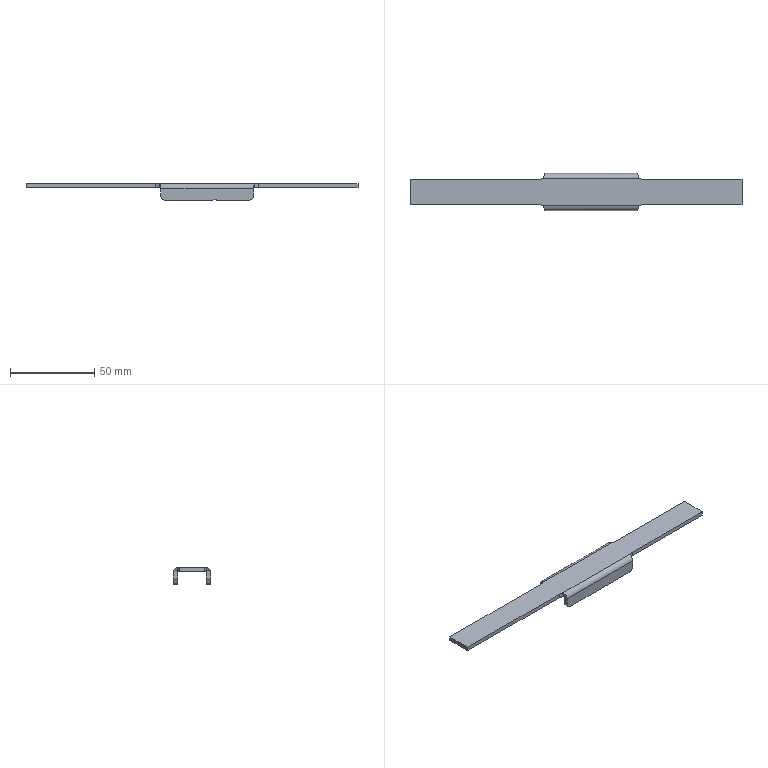Part | STEP file | lll_id4282_x_t | 1 solid | 44 faces | box 197 x 22 x 10 mm | volume 10197 mm3 | plane 24 | cylinder 20 | commonest cylinder face diameters 6 x18 1 x2
STEP:
#1=CARTESIAN_POINT('',(4075.236,8.5,-327.));
#2=VERTEX_POINT('',#1);
#3=CARTESIAN_POINT('',(4075.236,8.5,-324.542));
#4=VERTEX_POINT('',#3);
#5=CARTESIAN_POINT('',(4075.236,8.5,973.));
#6=DIRECTION('',(0.,0.,1.));
#7=VECTOR('',#6,1.);
#8=LINE('',#5,#7);
#9=EDGE_CURVE('',#2,#4,#8,.T.);
#10=ORIENTED_EDGE('',*,*,#9,.T.);
#11=CARTESIAN_POINT('',(4075.273,8.5,-324.542));
#12=VERTEX_POINT('',#11);
#13=CARTESIAN_POINT('',(4075.236,8.5,-324.542));
#14=DIRECTION('',(1.,0.,0.));
#15=VECTOR('',#14,1.);
#16=LINE('',#13,#15);
#17=EDGE_CURVE('',#4,#12,#16,.T.);
#18=ORIENTED_EDGE('',*,*,#17,.T.);
#19=CARTESIAN_POINT('',(4076.,8.5,-326.5));
#20=VERTEX_POINT('',#19);
#21=CARTESIAN_POINT('',(4073.,8.5,-326.5));
#22=DIRECTION('',(0.,1.,0.));
#23=DIRECTION('',(-1.,0.,0.));
#24=AXIS2_PLACEMENT_3D('',#21,#22,#23);
#25=CIRCLE('',#24,3.);
#26=EDGE_CURVE('',#12,#20,#25,.T.);
#27=ORIENTED_EDGE('',*,*,#26,.T.);
#28=CARTESIAN_POINT('',(4076.,8.5,-327.));
#29=VERTEX_POINT('',#28);
#30=CARTESIAN_POINT('',(4076.,8.5,-326.5));
#31=DIRECTION('',(0.,0.,-1.));
#32=VECTOR('',#31,1.);
#33=LINE('',#30,#32);
#34=EDGE_CURVE('',#20,#29,#33,.T.);
#35=ORIENTED_EDGE('',*,*,#34,.T.);
#36=CARTESIAN_POINT('',(14759.883,8.5,-327.));
#37=DIRECTION('',(1.,0.,0.));
#38=VECTOR('',#37,1.);
#39=LINE('',#36,#38);
#40=EDGE_CURVE('',#2,#29,#39,.T.);
#41=ORIENTED_EDGE('',*,*,#40,.F.);
#42=EDGE_LOOP('',(#10,#18,#27,#35,#41));
#43=FACE_OUTER_BOUND('',#42,.T.);
#44=CARTESIAN_POINT('',(4075.236,8.5,973.));
#45=DIRECTION('',(0.,1.,0.));
#46=DIRECTION('',(0.,0.,1.));
#47=AXIS2_PLACEMENT_3D('',#44,#45,#46);
#48=PLANE('',#47);
#49=ADVANCED_FACE('',(#43),#48,.T.);
#50=CARTESIAN_POINT('',(4131.764,-8.5,-327.));
#51=VERTEX_POINT('',#50);
#52=CARTESIAN_POINT('',(4131.764,-8.5,-324.542));
#53=VERTEX_POINT('',#52);
#54=CARTESIAN_POINT('',(4131.764,-8.5,973.));
#55=DIRECTION('',(0.,0.,1.));
#56=VECTOR('',#55,1.);
#57=LINE('',#54,#56);
#58=EDGE_CURVE('',#51,#53,#57,.T.);
#59=ORIENTED_EDGE('',*,*,#58,.T.);
#60=CARTESIAN_POINT('',(4131.727,-8.5,-324.542));
#61=VERTEX_POINT('',#60);
#62=CARTESIAN_POINT('',(4131.764,-8.5,-324.542));
#63=DIRECTION('',(-1.,0.,0.));
#64=VECTOR('',#63,1.);
#65=LINE('',#62,#64);
#66=EDGE_CURVE('',#53,#61,#65,.T.);
#67=ORIENTED_EDGE('',*,*,#66,.T.);
#68=CARTESIAN_POINT('',(4131.,-8.5,-326.5));
#69=VERTEX_POINT('',#68);
#70=CARTESIAN_POINT('',(4134.,-8.5,-326.5));
#71=DIRECTION('',(0.,-1.,0.));
#72=DIRECTION('',(-1.,0.,0.));
#73=AXIS2_PLACEMENT_3D('',#70,#71,#72);
#74=CIRCLE('',#73,3.);
#75=EDGE_CURVE('',#61,#69,#74,.T.);
#76=ORIENTED_EDGE('',*,*,#75,.T.);
#77=CARTESIAN_POINT('',(4131.,-8.5,-327.));
#78=VERTEX_POINT('',#77);
#79=CARTESIAN_POINT('',(4131.,-8.5,-326.5));
#80=DIRECTION('',(0.,0.,-1.));
#81=VECTOR('',#80,1.);
#82=LINE('',#79,#81);
#83=EDGE_CURVE('',#69,#78,#82,.T.);
#84=ORIENTED_EDGE('',*,*,#83,.T.);
#85=CARTESIAN_POINT('',(14759.883,-8.5,-327.));
#86=DIRECTION('',(1.,0.,0.));
#87=VECTOR('',#86,1.);
#88=LINE('',#85,#87);
#89=EDGE_CURVE('',#78,#51,#88,.T.);
#90=ORIENTED_EDGE('',*,*,#89,.T.);
#91=EDGE_LOOP('',(#59,#67,#76,#84,#90));
#92=FACE_OUTER_BOUND('',#91,.T.);
#93=CARTESIAN_POINT('',(4131.764,-8.5,973.));
#94=DIRECTION('',(0.,-1.,0.));
#95=DIRECTION('',(0.,0.,-1.));
#96=AXIS2_PLACEMENT_3D('',#93,#94,#95);
#97=PLANE('',#96);
#98=ADVANCED_FACE('',(#92),#97,.T.);
#99=CARTESIAN_POINT('',(4076.,-8.5,-326.5));
#100=VERTEX_POINT('',#99);
#101=CARTESIAN_POINT('',(4075.273,-8.5,-324.542));
#102=VERTEX_POINT('',#101);
#103=CARTESIAN_POINT('',(4073.,-8.5,-326.5));
#104=DIRECTION('',(0.,-1.,0.));
#105=DIRECTION('',(-1.,0.,0.));
#106=AXIS2_PLACEMENT_3D('',#103,#104,#105);
#107=CIRCLE('',#106,3.);
#108=EDGE_CURVE('',#100,#102,#107,.T.);
#109=ORIENTED_EDGE('',*,*,#108,.T.);
#110=CARTESIAN_POINT('',(4075.236,-8.5,-324.542));
#111=VERTEX_POINT('',#110);
#112=CARTESIAN_POINT('',(4075.273,-8.5,-324.542));
#113=DIRECTION('',(-1.,0.,0.));
#114=VECTOR('',#113,1.);
#115=LINE('',#112,#114);
#116=EDGE_CURVE('',#102,#111,#115,.T.);
#117=ORIENTED_EDGE('',*,*,#116,.T.);
#118=CARTESIAN_POINT('',(4075.236,-8.5,-327.));
#119=VERTEX_POINT('',#118);
#120=CARTESIAN_POINT('',(4075.236,-8.5,973.));
#121=DIRECTION('',(0.,0.,-1.));
#122=VECTOR('',#121,1.);
#123=LINE('',#120,#122);
#124=EDGE_CURVE('',#111,#119,#123,.T.);
#125=ORIENTED_EDGE('',*,*,#124,.T.);
#126=CARTESIAN_POINT('',(4076.,-8.5,-327.));
#127=VERTEX_POINT('',#126);
#128=CARTESIAN_POINT('',(14759.883,-8.5,-327.));
#129=DIRECTION('',(1.,0.,0.));
#130=VECTOR('',#129,1.);
#131=LINE('',#128,#130);
#132=EDGE_CURVE('',#119,#127,#131,.T.);
#133=ORIENTED_EDGE('',*,*,#132,.T.);
#134=CARTESIAN_POINT('',(4076.,-8.5,-331.5));
#135=DIRECTION('',(0.,0.,1.));
#136=VECTOR('',#135,1.);
#137=LINE('',#134,#136);
#138=EDGE_CURVE('',#127,#100,#137,.T.);
#139=ORIENTED_EDGE('',*,*,#138,.T.);
#140=EDGE_LOOP('',(#109,#117,#125,#133,#139));
#141=FACE_OUTER_BOUND('',#140,.T.);
#142=CARTESIAN_POINT('',(4131.764,-8.5,973.));
#143=DIRECTION('',(0.,-1.,0.));
#144=DIRECTION('',(0.,0.,-1.));
#145=AXIS2_PLACEMENT_3D('',#142,#143,#144);
#146=PLANE('',#145);
#147=ADVANCED_FACE('',(#141),#146,.T.);
#148=ORIENTED_EDGE('',*,*,#124,.F.);
#149=CARTESIAN_POINT('',(4074.658,-8.,-324.5));
#150=VERTEX_POINT('',#149);
#151=CARTESIAN_POINT('',(4075.236,-8.5,-324.542));
#152=CARTESIAN_POINT('',(4075.067,-8.311,-324.51));
#153=CARTESIAN_POINT('',(4074.871,-8.141,-324.5));
#154=CARTESIAN_POINT('',(4074.658,-8.,-324.5));
#155=B_SPLINE_CURVE_WITH_KNOTS('',3,(#151,#152,#153,#154),.UNSPECIFIED.,.F.,.F.,(4,4),(0.,1.),.UNSPECIFIED.);
#156=EDGE_CURVE('',#111,#150,#155,.T.);
#157=ORIENTED_EDGE('',*,*,#156,.T.);
#158=CARTESIAN_POINT('',(4073.,-7.5,-324.5));
#159=VERTEX_POINT('',#158);
#160=CARTESIAN_POINT('',(4073.,-10.5,-324.5));
#161=DIRECTION('',(0.,0.,1.));
#162=DIRECTION('',(-1.,0.,0.));
#163=AXIS2_PLACEMENT_3D('',#160,#161,#162);
#164=CIRCLE('',#163,3.);
#165=EDGE_CURVE('',#150,#159,#164,.T.);
#166=ORIENTED_EDGE('',*,*,#165,.T.);
#167=CARTESIAN_POINT('',(4073.,-7.5,-327.));
#168=VERTEX_POINT('',#167);
#169=CARTESIAN_POINT('',(4073.,-7.5,-324.5));
#170=DIRECTION('',(0.,0.,1.));
#171=VECTOR('',#170,1.);
#172=LINE('',#169,#171);
#173=EDGE_CURVE('',#168,#159,#172,.T.);
#174=ORIENTED_EDGE('',*,*,#173,.F.);
#175=CARTESIAN_POINT('',(4073.,-10.5,-327.));
#176=DIRECTION('',(0.,0.,1.));
#177=DIRECTION('',(-1.,0.,0.));
#178=AXIS2_PLACEMENT_3D('',#175,#176,#177);
#179=CIRCLE('',#178,3.);
#180=EDGE_CURVE('',#119,#168,#179,.T.);
#181=ORIENTED_EDGE('',*,*,#180,.F.);
#182=EDGE_LOOP('',(#148,#157,#166,#174,#181));
#183=FACE_OUTER_BOUND('',#182,.T.);
#184=CARTESIAN_POINT('',(4073.,-10.5,-324.5));
#185=DIRECTION('',(0.,0.,-1.));
#186=DIRECTION('',(-1.,0.,0.));
#187=AXIS2_PLACEMENT_3D('',#184,#185,#186);
#188=CYLINDRICAL_SURFACE('',#187,3.);
#189=ADVANCED_FACE('',(#183),#188,.F.);
#190=CARTESIAN_POINT('',(4134.,-7.5,-324.5));
#191=VERTEX_POINT('',#190);
#192=CARTESIAN_POINT('',(4132.342,-8.,-324.5));
#193=VERTEX_POINT('',#192);
#194=CARTESIAN_POINT('',(4134.,-10.5,-324.5));
#195=DIRECTION('',(0.,0.,1.));
#196=DIRECTION('',(-1.,0.,0.));
#197=AXIS2_PLACEMENT_3D('',#194,#195,#196);
#198=CIRCLE('',#197,3.);
#199=EDGE_CURVE('',#191,#193,#198,.T.);
#200=ORIENTED_EDGE('',*,*,#199,.T.);
#201=CARTESIAN_POINT('',(4132.342,-8.,-324.5));
#202=CARTESIAN_POINT('',(4132.129,-8.141,-324.5));
#203=CARTESIAN_POINT('',(4131.933,-8.311,-324.51));
#204=CARTESIAN_POINT('',(4131.764,-8.5,-324.542));
#205=B_SPLINE_CURVE_WITH_KNOTS('',3,(#201,#202,#203,#204),.UNSPECIFIED.,.F.,.F.,(4,4),(0.,1.),.UNSPECIFIED.);
#206=EDGE_CURVE('',#193,#53,#205,.T.);
#207=ORIENTED_EDGE('',*,*,#206,.T.);
#208=ORIENTED_EDGE('',*,*,#58,.F.);
#209=CARTESIAN_POINT('',(4134.,-7.5,-327.));
#210=VERTEX_POINT('',#209);
#211=CARTESIAN_POINT('',(4134.,-10.5,-327.));
#212=DIRECTION('',(0.,0.,1.));
#213=DIRECTION('',(-1.,0.,0.));
#214=AXIS2_PLACEMENT_3D('',#211,#212,#213);
#215=CIRCLE('',#214,3.);
#216=EDGE_CURVE('',#210,#51,#215,.T.);
#217=ORIENTED_EDGE('',*,*,#216,.F.);
#218=CARTESIAN_POINT('',(4134.,-7.5,-324.5));
#219=DIRECTION('',(0.,0.,1.));
#220=VECTOR('',#219,1.);
#221=LINE('',#218,#220);
#222=EDGE_CURVE('',#210,#191,#221,.T.);
#223=ORIENTED_EDGE('',*,*,#222,.T.);
#224=EDGE_LOOP('',(#200,#207,#208,#217,#223));
#225=FACE_OUTER_BOUND('',#224,.T.);
#226=CARTESIAN_POINT('',(4134.,-10.5,-324.5));
#227=DIRECTION('',(0.,0.,-1.));
#228=DIRECTION('',(-1.,0.,0.));
#229=AXIS2_PLACEMENT_3D('',#226,#227,#228);
#230=CYLINDRICAL_SURFACE('',#229,3.);
#231=ADVANCED_FACE('',(#225),#230,.F.);
#232=CARTESIAN_POINT('',(4193.,-7.5,-327.));
#233=VERTEX_POINT('',#232);
#234=CARTESIAN_POINT('',(4193.,7.5,-327.));
#235=VERTEX_POINT('',#234);
#236=CARTESIAN_POINT('',(4193.,-13712.786,-327.));
#237=DIRECTION('',(0.,1.,0.));
#238=VECTOR('',#237,1.);
#239=LINE('',#236,#238);
#240=EDGE_CURVE('',#233,#235,#239,.T.);
#241=ORIENTED_EDGE('',*,*,#240,.F.);
#242=CARTESIAN_POINT('',(4228.,-7.5,-327.));
#243=DIRECTION('',(-1.,0.,0.));
#244=VECTOR('',#243,1.);
#245=LINE('',#242,#244);
#246=EDGE_CURVE('',#233,#210,#245,.T.);
#247=ORIENTED_EDGE('',*,*,#246,.T.);
#248=ORIENTED_EDGE('',*,*,#216,.T.);
#249=ORIENTED_EDGE('',*,*,#89,.F.);
#250=CARTESIAN_POINT('',(4131.,-8.,-327.));
#251=VERTEX_POINT('',#250);
#252=CARTESIAN_POINT('',(4131.,-11.,-327.));
#253=DIRECTION('',(0.,1.,0.));
#254=VECTOR('',#253,1.);
#255=LINE('',#252,#254);
#256=EDGE_CURVE('',#78,#251,#255,.T.);
#257=ORIENTED_EDGE('',*,*,#256,.T.);
#258=CARTESIAN_POINT('',(4076.,-8.,-327.));
#259=VERTEX_POINT('',#258);
#260=CARTESIAN_POINT('',(4076.,-8.,-327.));
#261=DIRECTION('',(-1.,0.,0.));
#262=VECTOR('',#261,1.);
#263=LINE('',#260,#262);
#264=EDGE_CURVE('',#251,#259,#263,.T.);
#265=ORIENTED_EDGE('',*,*,#264,.T.);
#266=CARTESIAN_POINT('',(4076.,-11.,-327.));
#267=DIRECTION('',(0.,-1.,0.));
#268=VECTOR('',#267,1.);
#269=LINE('',#266,#268);
#270=EDGE_CURVE('',#259,#127,#269,.T.);
#271=ORIENTED_EDGE('',*,*,#270,.T.);
#272=ORIENTED_EDGE('',*,*,#132,.F.);
#273=ORIENTED_EDGE('',*,*,#180,.T.);
#274=CARTESIAN_POINT('',(3996.,-7.5,-327.));
#275=VERTEX_POINT('',#274);
#276=CARTESIAN_POINT('',(4073.,-7.5,-327.));
#277=DIRECTION('',(-1.,0.,0.));
#278=VECTOR('',#277,1.);
#279=LINE('',#276,#278);
#280=EDGE_CURVE('',#168,#275,#279,.T.);
#281=ORIENTED_EDGE('',*,*,#280,.T.);
#282=CARTESIAN_POINT('',(3996.,7.5,-327.));
#283=VERTEX_POINT('',#282);
#284=CARTESIAN_POINT('',(3996.,-13712.786,-327.));
#285=DIRECTION('',(0.,1.,0.));
#286=VECTOR('',#285,1.);
#287=LINE('',#284,#286);
#288=EDGE_CURVE('',#275,#283,#287,.T.);
#289=ORIENTED_EDGE('',*,*,#288,.T.);
#290=CARTESIAN_POINT('',(4073.,7.5,-327.));
#291=VERTEX_POINT('',#290);
#292=CARTESIAN_POINT('',(3991.,7.5,-327.));
#293=DIRECTION('',(1.,0.,0.));
#294=VECTOR('',#293,1.);
#295=LINE('',#292,#294);
#296=EDGE_CURVE('',#283,#291,#295,.T.);
#297=ORIENTED_EDGE('',*,*,#296,.T.);
#298=CARTESIAN_POINT('',(4073.,10.5,-327.));
#299=DIRECTION('',(0.,0.,1.));
#300=DIRECTION('',(-1.,0.,0.));
#301=AXIS2_PLACEMENT_3D('',#298,#299,#300);
#302=CIRCLE('',#301,3.);
#303=EDGE_CURVE('',#291,#2,#302,.T.);
#304=ORIENTED_EDGE('',*,*,#303,.T.);
#305=ORIENTED_EDGE('',*,*,#40,.T.);
#306=CARTESIAN_POINT('',(4076.,8.,-327.));
#307=VERTEX_POINT('',#306);
#308=CARTESIAN_POINT('',(4076.,11.,-327.));
#309=DIRECTION('',(0.,-1.,0.));
#310=VECTOR('',#309,1.);
#311=LINE('',#308,#310);
#312=EDGE_CURVE('',#29,#307,#311,.T.);
#313=ORIENTED_EDGE('',*,*,#312,.T.);
#314=CARTESIAN_POINT('',(4131.,8.,-327.));
#315=VERTEX_POINT('',#314);
#316=CARTESIAN_POINT('',(4131.,8.,-327.));
#317=DIRECTION('',(1.,0.,0.));
#318=VECTOR('',#317,1.);
#319=LINE('',#316,#318);
#320=EDGE_CURVE('',#307,#315,#319,.T.);
#321=ORIENTED_EDGE('',*,*,#320,.T.);
#322=CARTESIAN_POINT('',(4131.,8.5,-327.));
#323=VERTEX_POINT('',#322);
#324=CARTESIAN_POINT('',(4131.,-13712.786,-327.));
#325=DIRECTION('',(0.,1.,0.));
#326=VECTOR('',#325,1.);
#327=LINE('',#324,#326);
#328=EDGE_CURVE('',#315,#323,#327,.T.);
#329=ORIENTED_EDGE('',*,*,#328,.T.);
#330=CARTESIAN_POINT('',(4131.764,8.5,-327.));
#331=VERTEX_POINT('',#330);
#332=CARTESIAN_POINT('',(14759.883,8.5,-327.));
#333=DIRECTION('',(1.,0.,0.));
#334=VECTOR('',#333,1.);
#335=LINE('',#332,#334);
#336=EDGE_CURVE('',#323,#331,#335,.T.);
#337=ORIENTED_EDGE('',*,*,#336,.T.);
#338=CARTESIAN_POINT('',(4134.,7.5,-327.));
#339=VERTEX_POINT('',#338);
#340=CARTESIAN_POINT('',(4134.,10.5,-327.));
#341=DIRECTION('',(0.,0.,-1.));
#342=DIRECTION('',(-1.,0.,0.));
#343=AXIS2_PLACEMENT_3D('',#340,#341,#342);
#344=CIRCLE('',#343,3.);
#345=EDGE_CURVE('',#339,#331,#344,.T.);
#346=ORIENTED_EDGE('',*,*,#345,.F.);
#347=CARTESIAN_POINT('',(4228.,7.5,-327.));
#348=DIRECTION('',(-1.,0.,0.));
#349=VECTOR('',#348,1.);
#350=LINE('',#347,#349);
#351=EDGE_CURVE('',#235,#339,#350,.T.);
#352=ORIENTED_EDGE('',*,*,#351,.F.);
#353=EDGE_LOOP('',(#241,#247,#248,#249,#257,#265,#271,#272,#273,#281,#289,#297,#304,#305,#313,#321,#329,#337,#346,#352));
#354=FACE_OUTER_BOUND('',#353,.T.);
#355=CARTESIAN_POINT('',(14759.883,-13712.786,-327.));
#356=DIRECTION('',(0.,0.,-1.));
#357=DIRECTION('',(-1.,0.,0.));
#358=AXIS2_PLACEMENT_3D('',#355,#356,#357);
#359=PLANE('',#358);
#360=ADVANCED_FACE('',(#354),#359,.T.);
#361=CARTESIAN_POINT('',(4193.,-7.5,-324.5));
#362=VERTEX_POINT('',#361);
#363=CARTESIAN_POINT('',(4228.,-7.5,-324.5));
#364=DIRECTION('',(-1.,0.,0.));
#365=VECTOR('',#364,1.);
#366=LINE('',#363,#365);
#367=EDGE_CURVE('',#362,#191,#366,.T.);
#368=ORIENTED_EDGE('',*,*,#367,.F.);
#369=CARTESIAN_POINT('',(4193.,7.5,-324.5));
#370=VERTEX_POINT('',#369);
#371=CARTESIAN_POINT('',(4193.,-13712.786,-324.5));
#372=DIRECTION('',(0.,-1.,0.));
#373=VECTOR('',#372,1.);
#374=LINE('',#371,#373);
#375=EDGE_CURVE('',#370,#362,#374,.T.);
#376=ORIENTED_EDGE('',*,*,#375,.F.);
#377=CARTESIAN_POINT('',(4134.,7.5,-324.5));
#378=VERTEX_POINT('',#377);
#379=CARTESIAN_POINT('',(4228.,7.5,-324.5));
#380=DIRECTION('',(-1.,0.,0.));
#381=VECTOR('',#380,1.);
#382=LINE('',#379,#381);
#383=EDGE_CURVE('',#370,#378,#382,.T.);
#384=ORIENTED_EDGE('',*,*,#383,.T.);
#385=CARTESIAN_POINT('',(4132.342,8.,-324.5));
#386=VERTEX_POINT('',#385);
#387=CARTESIAN_POINT('',(4134.,10.5,-324.5));
#388=DIRECTION('',(0.,0.,-1.));
#389=DIRECTION('',(-1.,0.,0.));
#390=AXIS2_PLACEMENT_3D('',#387,#388,#389);
#391=CIRCLE('',#390,3.);
#392=EDGE_CURVE('',#378,#386,#391,.T.);
#393=ORIENTED_EDGE('',*,*,#392,.T.);
#394=CARTESIAN_POINT('',(4074.658,8.,-324.5));
#395=VERTEX_POINT('',#394);
#396=CARTESIAN_POINT('',(14759.883,8.,-324.5));
#397=DIRECTION('',(-1.,0.,0.));
#398=VECTOR('',#397,1.);
#399=LINE('',#396,#398);
#400=EDGE_CURVE('',#386,#395,#399,.T.);
#401=ORIENTED_EDGE('',*,*,#400,.T.);
#402=CARTESIAN_POINT('',(4073.,7.5,-324.5));
#403=VERTEX_POINT('',#402);
#404=CARTESIAN_POINT('',(4073.,10.5,-324.5));
#405=DIRECTION('',(0.,0.,1.));
#406=DIRECTION('',(-1.,0.,0.));
#407=AXIS2_PLACEMENT_3D('',#404,#405,#406);
#408=CIRCLE('',#407,3.);
#409=EDGE_CURVE('',#403,#395,#408,.T.);
#410=ORIENTED_EDGE('',*,*,#409,.F.);
#411=CARTESIAN_POINT('',(3996.,7.5,-324.5));
#412=VERTEX_POINT('',#411);
#413=CARTESIAN_POINT('',(3991.,7.5,-324.5));
#414=DIRECTION('',(1.,0.,0.));
#415=VECTOR('',#414,1.);
#416=LINE('',#413,#415);
#417=EDGE_CURVE('',#412,#403,#416,.T.);
#418=ORIENTED_EDGE('',*,*,#417,.F.);
#419=CARTESIAN_POINT('',(3996.,-7.5,-324.5));
#420=VERTEX_POINT('',#419);
#421=CARTESIAN_POINT('',(3996.,-13712.786,-324.5));
#422=DIRECTION('',(0.,1.,0.));
#423=VECTOR('',#422,1.);
#424=LINE('',#421,#423);
#425=EDGE_CURVE('',#420,#412,#424,.T.);
#426=ORIENTED_EDGE('',*,*,#425,.F.);
#427=CARTESIAN_POINT('',(4073.,-7.5,-324.5));
#428=DIRECTION('',(-1.,0.,0.));
#429=VECTOR('',#428,1.);
#430=LINE('',#427,#429);
#431=EDGE_CURVE('',#159,#420,#430,.T.);
#432=ORIENTED_EDGE('',*,*,#431,.F.);
#433=ORIENTED_EDGE('',*,*,#165,.F.);
#434=CARTESIAN_POINT('',(14759.883,-8.,-324.5));
#435=DIRECTION('',(1.,0.,0.));
#436=VECTOR('',#435,1.);
#437=LINE('',#434,#436);
#438=EDGE_CURVE('',#150,#193,#437,.T.);
#439=ORIENTED_EDGE('',*,*,#438,.T.);
#440=ORIENTED_EDGE('',*,*,#199,.F.);
#441=EDGE_LOOP('',(#368,#376,#384,#393,#401,#410,#418,#426,#432,#433,#439,#440));
#442=FACE_OUTER_BOUND('',#441,.T.);
#443=CARTESIAN_POINT('',(14759.883,-13712.786,-324.5));
#444=DIRECTION('',(0.,0.,-1.));
#445=DIRECTION('',(-1.,0.,0.));
#446=AXIS2_PLACEMENT_3D('',#443,#444,#445);
#447=PLANE('',#446);
#448=ADVANCED_FACE('',(#442),#447,.F.);
#449=ORIENTED_EDGE('',*,*,#296,.F.);
#450=CARTESIAN_POINT('',(3996.,7.5,-324.5));
#451=DIRECTION('',(0.,0.,-1.));
#452=VECTOR('',#451,1.);
#453=LINE('',#450,#452);
#454=EDGE_CURVE('',#412,#283,#453,.T.);
#455=ORIENTED_EDGE('',*,*,#454,.F.);
#456=ORIENTED_EDGE('',*,*,#417,.T.);
#457=CARTESIAN_POINT('',(4073.,7.5,-324.5));
#458=DIRECTION('',(0.,0.,1.));
#459=VECTOR('',#458,1.);
#460=LINE('',#457,#459);
#461=EDGE_CURVE('',#291,#403,#460,.T.);
#462=ORIENTED_EDGE('',*,*,#461,.F.);
#463=EDGE_LOOP('',(#449,#455,#456,#462));
#464=FACE_OUTER_BOUND('',#463,.T.);
#465=CARTESIAN_POINT('',(3991.,7.5,-324.5));
#466=DIRECTION('',(0.,1.,0.));
#467=DIRECTION('',(0.,0.,1.));
#468=AXIS2_PLACEMENT_3D('',#465,#466,#467);
#469=PLANE('',#468);
#470=ADVANCED_FACE('',(#464),#469,.T.);
#471=CARTESIAN_POINT('',(3996.,-7.5,-1629.5));
#472=DIRECTION('',(0.,0.,1.));
#473=VECTOR('',#472,1.);
#474=LINE('',#471,#473);
#475=EDGE_CURVE('',#275,#420,#474,.T.);
#476=ORIENTED_EDGE('',*,*,#475,.T.);
#477=ORIENTED_EDGE('',*,*,#425,.T.);
#478=ORIENTED_EDGE('',*,*,#454,.T.);
#479=ORIENTED_EDGE('',*,*,#288,.F.);
#480=EDGE_LOOP('',(#476,#477,#478,#479));
#481=FACE_OUTER_BOUND('',#480,.T.);
#482=CARTESIAN_POINT('',(3996.,29.64,-1629.5));
#483=DIRECTION('',(-1.,0.,0.));
#484=DIRECTION('',(0.,0.,1.));
#485=AXIS2_PLACEMENT_3D('',#482,#483,#484);
#486=PLANE('',#485);
#487=ADVANCED_FACE('',(#481),#486,.T.);
#488=ORIENTED_EDGE('',*,*,#431,.T.);
#489=ORIENTED_EDGE('',*,*,#475,.F.);
#490=ORIENTED_EDGE('',*,*,#280,.F.);
#491=ORIENTED_EDGE('',*,*,#173,.T.);
#492=EDGE_LOOP('',(#488,#489,#490,#491));
#493=FACE_OUTER_BOUND('',#492,.T.);
#494=CARTESIAN_POINT('',(4073.,-7.5,-324.5));
#495=DIRECTION('',(0.,-1.,0.));
#496=DIRECTION('',(0.,0.,-1.));
#497=AXIS2_PLACEMENT_3D('',#494,#495,#496);
#498=PLANE('',#497);
#499=ADVANCED_FACE('',(#493),#498,.T.);
#500=CARTESIAN_POINT('',(4193.,-7.5,-324.5));
#501=DIRECTION('',(0.,0.,1.));
#502=VECTOR('',#501,1.);
#503=LINE('',#500,#502);
#504=EDGE_CURVE('',#233,#362,#503,.T.);
#505=ORIENTED_EDGE('',*,*,#504,.T.);
#506=ORIENTED_EDGE('',*,*,#367,.T.);
#507=ORIENTED_EDGE('',*,*,#222,.F.);
#508=ORIENTED_EDGE('',*,*,#246,.F.);
#509=EDGE_LOOP('',(#505,#506,#507,#508));
#510=FACE_OUTER_BOUND('',#509,.T.);
#511=CARTESIAN_POINT('',(4228.,-7.5,-324.5));
#512=DIRECTION('',(0.,-1.,0.));
#513=DIRECTION('',(-1.,0.,0.));
#514=AXIS2_PLACEMENT_3D('',#511,#512,#513);
#515=PLANE('',#514);
#516=ADVANCED_FACE('',(#510),#515,.T.);
#517=ORIENTED_EDGE('',*,*,#383,.F.);
#518=CARTESIAN_POINT('',(4193.,7.5,-324.5));
#519=DIRECTION('',(0.,0.,-1.));
#520=VECTOR('',#519,1.);
#521=LINE('',#518,#520);
#522=EDGE_CURVE('',#370,#235,#521,.T.);
#523=ORIENTED_EDGE('',*,*,#522,.T.);
#524=ORIENTED_EDGE('',*,*,#351,.T.);
#525=CARTESIAN_POINT('',(4134.,7.5,-324.5));
#526=DIRECTION('',(0.,0.,1.));
#527=VECTOR('',#526,1.);
#528=LINE('',#525,#527);
#529=EDGE_CURVE('',#339,#378,#528,.T.);
#530=ORIENTED_EDGE('',*,*,#529,.T.);
#531=EDGE_LOOP('',(#517,#523,#524,#530));
#532=FACE_OUTER_BOUND('',#531,.T.);
#533=CARTESIAN_POINT('',(4228.,7.5,-324.5));
#534=DIRECTION('',(0.,-1.,0.));
#535=DIRECTION('',(-1.,0.,0.));
#536=AXIS2_PLACEMENT_3D('',#533,#534,#535);
#537=PLANE('',#536);
#538=ADVANCED_FACE('',(#532),#537,.F.);
#539=CARTESIAN_POINT('',(4131.764,8.5,-324.542));
#540=VERTEX_POINT('',#539);
#541=CARTESIAN_POINT('',(4131.764,8.5,973.));
#542=DIRECTION('',(0.,0.,-1.));
#543=VECTOR('',#542,1.);
#544=LINE('',#541,#543);
#545=EDGE_CURVE('',#540,#331,#544,.T.);
#546=ORIENTED_EDGE('',*,*,#545,.F.);
#547=CARTESIAN_POINT('',(4131.764,8.5,-324.542));
#548=CARTESIAN_POINT('',(4131.933,8.311,-324.51));
#549=CARTESIAN_POINT('',(4132.129,8.141,-324.5));
#550=CARTESIAN_POINT('',(4132.342,8.,-324.5));
#551=B_SPLINE_CURVE_WITH_KNOTS('',3,(#547,#548,#549,#550),.UNSPECIFIED.,.F.,.F.,(4,4),(0.,1.),.UNSPECIFIED.);
#552=EDGE_CURVE('',#540,#386,#551,.T.);
#553=ORIENTED_EDGE('',*,*,#552,.T.);
#554=ORIENTED_EDGE('',*,*,#392,.F.);
#555=ORIENTED_EDGE('',*,*,#529,.F.);
#556=ORIENTED_EDGE('',*,*,#345,.T.);
#557=EDGE_LOOP('',(#546,#553,#554,#555,#556));
#558=FACE_OUTER_BOUND('',#557,.T.);
#559=CARTESIAN_POINT('',(4134.,10.5,-324.5));
#560=DIRECTION('',(0.,0.,-1.));
#561=DIRECTION('',(-1.,0.,0.));
#562=AXIS2_PLACEMENT_3D('',#559,#560,#561);
#563=CYLINDRICAL_SURFACE('',#562,3.);
#564=ADVANCED_FACE('',(#558),#563,.F.);
#565=ORIENTED_EDGE('',*,*,#409,.T.);
#566=CARTESIAN_POINT('',(4074.658,8.,-324.5));
#567=CARTESIAN_POINT('',(4074.871,8.141,-324.5));
#568=CARTESIAN_POINT('',(4075.067,8.311,-324.51));
#569=CARTESIAN_POINT('',(4075.236,8.5,-324.542));
#570=B_SPLINE_CURVE_WITH_KNOTS('',3,(#566,#567,#568,#569),.UNSPECIFIED.,.F.,.F.,(4,4),(0.,1.),.UNSPECIFIED.);
#571=EDGE_CURVE('',#395,#4,#570,.T.);
#572=ORIENTED_EDGE('',*,*,#571,.T.);
#573=ORIENTED_EDGE('',*,*,#9,.F.);
#574=ORIENTED_EDGE('',*,*,#303,.F.);
#575=ORIENTED_EDGE('',*,*,#461,.T.);
#576=EDGE_LOOP('',(#565,#572,#573,#574,#575));
#577=FACE_OUTER_BOUND('',#576,.T.);
#578=CARTESIAN_POINT('',(4073.,10.5,-324.5));
#579=DIRECTION('',(0.,0.,-1.));
#580=DIRECTION('',(-1.,0.,0.));
#581=AXIS2_PLACEMENT_3D('',#578,#579,#580);
#582=CYLINDRICAL_SURFACE('',#581,3.);
#583=ADVANCED_FACE('',(#577),#582,.F.);
#584=CARTESIAN_POINT('',(4131.727,8.5,-324.542));
#585=VERTEX_POINT('',#584);
#586=CARTESIAN_POINT('',(4131.,8.5,-326.5));
#587=VERTEX_POINT('',#586);
#588=CARTESIAN_POINT('',(4134.,8.5,-326.5));
#589=DIRECTION('',(0.,-1.,0.));
#590=DIRECTION('',(-1.,0.,0.));
#591=AXIS2_PLACEMENT_3D('',#588,#589,#590);
#592=CIRCLE('',#591,3.);
#593=EDGE_CURVE('',#585,#587,#592,.T.);
#594=ORIENTED_EDGE('',*,*,#593,.F.);
#595=CARTESIAN_POINT('',(4131.727,8.5,-324.542));
#596=DIRECTION('',(1.,0.,0.));
#597=VECTOR('',#596,1.);
#598=LINE('',#595,#597);
#599=EDGE_CURVE('',#585,#540,#598,.T.);
#600=ORIENTED_EDGE('',*,*,#599,.T.);
#601=ORIENTED_EDGE('',*,*,#545,.T.);
#602=ORIENTED_EDGE('',*,*,#336,.F.);
#603=CARTESIAN_POINT('',(4131.,8.5,-326.5));
#604=DIRECTION('',(0.,0.,-1.));
#605=VECTOR('',#604,1.);
#606=LINE('',#603,#605);
#607=EDGE_CURVE('',#587,#323,#606,.T.);
#608=ORIENTED_EDGE('',*,*,#607,.F.);
#609=EDGE_LOOP('',(#594,#600,#601,#602,#608));
#610=FACE_OUTER_BOUND('',#609,.T.);
#611=CARTESIAN_POINT('',(4075.236,8.5,973.));
#612=DIRECTION('',(0.,1.,0.));
#613=DIRECTION('',(0.,0.,1.));
#614=AXIS2_PLACEMENT_3D('',#611,#612,#613);
#615=PLANE('',#614);
#616=ADVANCED_FACE('',(#610),#615,.T.);
#617=CARTESIAN_POINT('',(4131.,-10.828,-326.5));
#618=VERTEX_POINT('',#617);
#619=CARTESIAN_POINT('',(4131.,-11.,-326.5));
#620=DIRECTION('',(0.,-1.,0.));
#621=VECTOR('',#620,1.);
#622=LINE('',#619,#621);
#623=EDGE_CURVE('',#69,#618,#622,.T.);
#624=ORIENTED_EDGE('',*,*,#623,.T.);
#625=CARTESIAN_POINT('',(4131.,-11.,-327.5));
#626=VERTEX_POINT('',#625);
#627=CARTESIAN_POINT('',(4131.,-8.,-327.5));
#628=DIRECTION('',(1.,0.,0.));
#629=DIRECTION('',(0.,0.,1.));
#630=AXIS2_PLACEMENT_3D('',#627,#628,#629);
#631=CIRCLE('',#630,3.);
#632=EDGE_CURVE('',#618,#626,#631,.T.);
#633=ORIENTED_EDGE('',*,*,#632,.T.);
#634=CARTESIAN_POINT('',(4131.,-11.,-331.5));
#635=VERTEX_POINT('',#634);
#636=CARTESIAN_POINT('',(4131.,-11.,-326.5));
#637=DIRECTION('',(0.,0.,-1.));
#638=VECTOR('',#637,1.);
#639=LINE('',#636,#638);
#640=EDGE_CURVE('',#626,#635,#639,.T.);
#641=ORIENTED_EDGE('',*,*,#640,.T.);
#642=CARTESIAN_POINT('',(4131.,-8.5,-331.5));
#643=VERTEX_POINT('',#642);
#644=CARTESIAN_POINT('',(4131.,-11.,-331.5));
#645=DIRECTION('',(0.,-1.,0.));
#646=VECTOR('',#645,1.);
#647=LINE('',#644,#646);
#648=EDGE_CURVE('',#643,#635,#647,.T.);
#649=ORIENTED_EDGE('',*,*,#648,.F.);
#650=CARTESIAN_POINT('',(4131.,-8.5,-327.5));
#651=VERTEX_POINT('',#650);
#652=CARTESIAN_POINT('',(4131.,-8.5,-326.5));
#653=DIRECTION('',(0.,0.,-1.));
#654=VECTOR('',#653,1.);
#655=LINE('',#652,#654);
#656=EDGE_CURVE('',#651,#643,#655,.T.);
#657=ORIENTED_EDGE('',*,*,#656,.F.);
#658=CARTESIAN_POINT('',(4131.,-8.,-327.5));
#659=DIRECTION('',(-1.,0.,0.));
#660=DIRECTION('',(0.,0.,1.));
#661=AXIS2_PLACEMENT_3D('',#658,#659,#660);
#662=CIRCLE('',#661,0.5);
#663=EDGE_CURVE('',#651,#251,#662,.T.);
#664=ORIENTED_EDGE('',*,*,#663,.T.);
#665=ORIENTED_EDGE('',*,*,#256,.F.);
#666=ORIENTED_EDGE('',*,*,#83,.F.);
#667=EDGE_LOOP('',(#624,#633,#641,#649,#657,#664,#665,#666));
#668=FACE_OUTER_BOUND('',#667,.T.);
#669=CARTESIAN_POINT('',(4131.,-11.,-326.5));
#670=DIRECTION('',(1.,0.,0.));
#671=DIRECTION('',(0.,1.,0.));
#672=AXIS2_PLACEMENT_3D('',#669,#670,#671);
#673=PLANE('',#672);
#674=ADVANCED_FACE('',(#668),#673,.T.);
#675=CARTESIAN_POINT('',(4128.,-8.5,-334.5));
#676=VERTEX_POINT('',#675);
#677=CARTESIAN_POINT('',(4128.,-8.5,-331.5));
#678=DIRECTION('',(0.,1.,0.));
#679=DIRECTION('',(-1.,0.,0.));
#680=AXIS2_PLACEMENT_3D('',#677,#678,#679);
#681=CIRCLE('',#680,3.);
#682=EDGE_CURVE('',#643,#676,#681,.T.);
#683=ORIENTED_EDGE('',*,*,#682,.F.);
#684=ORIENTED_EDGE('',*,*,#648,.T.);
#685=CARTESIAN_POINT('',(4128.,-11.,-334.5));
#686=VERTEX_POINT('',#685);
#687=CARTESIAN_POINT('',(4128.,-11.,-331.5));
#688=DIRECTION('',(0.,1.,0.));
#689=DIRECTION('',(-1.,0.,0.));
#690=AXIS2_PLACEMENT_3D('',#687,#688,#689);
#691=CIRCLE('',#690,3.);
#692=EDGE_CURVE('',#635,#686,#691,.T.);
#693=ORIENTED_EDGE('',*,*,#692,.T.);
#694=CARTESIAN_POINT('',(4128.,-11.,-334.5));
#695=DIRECTION('',(0.,-1.,0.));
#696=VECTOR('',#695,1.);
#697=LINE('',#694,#696);
#698=EDGE_CURVE('',#676,#686,#697,.T.);
#699=ORIENTED_EDGE('',*,*,#698,.F.);
#700=EDGE_LOOP('',(#683,#684,#693,#699));
#701=FACE_OUTER_BOUND('',#700,.T.);
#702=CARTESIAN_POINT('',(4128.,-11.,-331.5));
#703=DIRECTION('',(0.,1.,0.));
#704=DIRECTION('',(-1.,0.,0.));
#705=AXIS2_PLACEMENT_3D('',#702,#703,#704);
#706=CYLINDRICAL_SURFACE('',#705,3.);
#707=ADVANCED_FACE('',(#701),#706,.T.);
#708=CARTESIAN_POINT('',(4109.658,-8.5,-334.5));
#709=VERTEX_POINT('',#708);
#710=CARTESIAN_POINT('',(4128.,-8.5,-334.5));
#711=DIRECTION('',(-1.,0.,0.));
#712=VECTOR('',#711,1.);
#713=LINE('',#710,#712);
#714=EDGE_CURVE('',#676,#709,#713,.T.);
#715=ORIENTED_EDGE('',*,*,#714,.F.);
#716=ORIENTED_EDGE('',*,*,#698,.T.);
#717=CARTESIAN_POINT('',(4109.658,-11.,-334.5));
#718=VERTEX_POINT('',#717);
#719=CARTESIAN_POINT('',(4128.,-11.,-334.5));
#720=DIRECTION('',(-1.,0.,0.));
#721=VECTOR('',#720,1.);
#722=LINE('',#719,#721);
#723=EDGE_CURVE('',#686,#718,#722,.T.);
#724=ORIENTED_EDGE('',*,*,#723,.T.);
#725=CARTESIAN_POINT('',(4109.658,-11.,-334.5));
#726=DIRECTION('',(0.,-1.,0.));
#727=VECTOR('',#726,1.);
#728=LINE('',#725,#727);
#729=EDGE_CURVE('',#709,#718,#728,.T.);
#730=ORIENTED_EDGE('',*,*,#729,.F.);
#731=EDGE_LOOP('',(#715,#716,#724,#730));
#732=FACE_OUTER_BOUND('',#731,.T.);
#733=CARTESIAN_POINT('',(4128.,-11.,-334.5));
#734=DIRECTION('',(0.,0.,-1.));
#735=DIRECTION('',(0.,1.,0.));
#736=AXIS2_PLACEMENT_3D('',#733,#734,#735);
#737=PLANE('',#736);
#738=ADVANCED_FACE('',(#732),#737,.T.);
#739=CARTESIAN_POINT('',(4106.801,-8.5,-334.25));
#740=VERTEX_POINT('',#739);
#741=CARTESIAN_POINT('',(4108.,-8.5,-337.));
#742=DIRECTION('',(0.,-1.,0.));
#743=DIRECTION('',(-1.,0.,0.));
#744=AXIS2_PLACEMENT_3D('',#741,#742,#743);
#745=CIRCLE('',#744,3.);
#746=EDGE_CURVE('',#709,#740,#745,.T.);
#747=ORIENTED_EDGE('',*,*,#746,.F.);
#748=ORIENTED_EDGE('',*,*,#729,.T.);
#749=CARTESIAN_POINT('',(4106.801,-11.,-334.25));
#750=VERTEX_POINT('',#749);
#751=CARTESIAN_POINT('',(4108.,-11.,-337.));
#752=DIRECTION('',(0.,-1.,0.));
#753=DIRECTION('',(-1.,0.,0.));
#754=AXIS2_PLACEMENT_3D('',#751,#752,#753);
#755=CIRCLE('',#754,3.);
#756=EDGE_CURVE('',#718,#750,#755,.T.);
#757=ORIENTED_EDGE('',*,*,#756,.T.);
#758=CARTESIAN_POINT('',(4106.801,-11.,-334.25));
#759=DIRECTION('',(0.,-1.,0.));
#760=VECTOR('',#759,1.);
#761=LINE('',#758,#760);
#762=EDGE_CURVE('',#740,#750,#761,.T.);
#763=ORIENTED_EDGE('',*,*,#762,.F.);
#764=EDGE_LOOP('',(#747,#748,#757,#763));
#765=FACE_OUTER_BOUND('',#764,.T.);
#766=CARTESIAN_POINT('',(4108.,-11.,-337.));
#767=DIRECTION('',(0.,1.,0.));
#768=DIRECTION('',(-1.,0.,0.));
#769=AXIS2_PLACEMENT_3D('',#766,#767,#768);
#770=CYLINDRICAL_SURFACE('',#769,3.);
#771=ADVANCED_FACE('',(#765),#770,.F.);
#772=CARTESIAN_POINT('',(4105.602,-8.5,-334.5));
#773=VERTEX_POINT('',#772);
#774=CARTESIAN_POINT('',(4105.602,-8.5,-331.5));
#775=DIRECTION('',(0.,1.,0.));
#776=DIRECTION('',(-1.,0.,0.));
#777=AXIS2_PLACEMENT_3D('',#774,#775,#776);
#778=CIRCLE('',#777,3.);
#779=EDGE_CURVE('',#740,#773,#778,.T.);
#780=ORIENTED_EDGE('',*,*,#779,.F.);
#781=ORIENTED_EDGE('',*,*,#762,.T.);
#782=CARTESIAN_POINT('',(4105.602,-11.,-334.5));
#783=VERTEX_POINT('',#782);
#784=CARTESIAN_POINT('',(4105.602,-11.,-331.5));
#785=DIRECTION('',(0.,1.,0.));
#786=DIRECTION('',(-1.,0.,0.));
#787=AXIS2_PLACEMENT_3D('',#784,#785,#786);
#788=CIRCLE('',#787,3.);
#789=EDGE_CURVE('',#750,#783,#788,.T.);
#790=ORIENTED_EDGE('',*,*,#789,.T.);
#791=CARTESIAN_POINT('',(4105.602,-11.,-334.5));
#792=DIRECTION('',(0.,-1.,0.));
#793=VECTOR('',#792,1.);
#794=LINE('',#791,#793);
#795=EDGE_CURVE('',#773,#783,#794,.T.);
#796=ORIENTED_EDGE('',*,*,#795,.F.);
#797=EDGE_LOOP('',(#780,#781,#790,#796));
#798=FACE_OUTER_BOUND('',#797,.T.);
#799=CARTESIAN_POINT('',(4105.602,-11.,-331.5));
#800=DIRECTION('',(0.,1.,0.));
#801=DIRECTION('',(-1.,0.,0.));
#802=AXIS2_PLACEMENT_3D('',#799,#800,#801);
#803=CYLINDRICAL_SURFACE('',#802,3.);
#804=ADVANCED_FACE('',(#798),#803,.T.);
#805=CARTESIAN_POINT('',(4079.,-8.5,-334.5));
#806=VERTEX_POINT('',#805);
#807=CARTESIAN_POINT('',(4105.602,-8.5,-334.5));
#808=DIRECTION('',(-1.,0.,0.));
#809=VECTOR('',#808,1.);
#810=LINE('',#807,#809);
#811=EDGE_CURVE('',#773,#806,#810,.T.);
#812=ORIENTED_EDGE('',*,*,#811,.F.);
#813=ORIENTED_EDGE('',*,*,#795,.T.);
#814=CARTESIAN_POINT('',(4079.,-11.,-334.5));
#815=VERTEX_POINT('',#814);
#816=CARTESIAN_POINT('',(4105.602,-11.,-334.5));
#817=DIRECTION('',(-1.,0.,0.));
#818=VECTOR('',#817,1.);
#819=LINE('',#816,#818);
#820=EDGE_CURVE('',#783,#815,#819,.T.);
#821=ORIENTED_EDGE('',*,*,#820,.T.);
#822=CARTESIAN_POINT('',(4079.,-11.,-334.5));
#823=DIRECTION('',(0.,-1.,0.));
#824=VECTOR('',#823,1.);
#825=LINE('',#822,#824);
#826=EDGE_CURVE('',#806,#815,#825,.T.);
#827=ORIENTED_EDGE('',*,*,#826,.F.);
#828=EDGE_LOOP('',(#812,#813,#821,#827));
#829=FACE_OUTER_BOUND('',#828,.T.);
#830=CARTESIAN_POINT('',(4105.602,-11.,-334.5));
#831=DIRECTION('',(0.,0.,-1.));
#832=DIRECTION('',(0.,1.,0.));
#833=AXIS2_PLACEMENT_3D('',#830,#831,#832);
#834=PLANE('',#833);
#835=ADVANCED_FACE('',(#829),#834,.T.);
#836=CARTESIAN_POINT('',(4076.,-8.5,-331.5));
#837=VERTEX_POINT('',#836);
#838=CARTESIAN_POINT('',(4079.,-8.5,-331.5));
#839=DIRECTION('',(0.,1.,0.));
#840=DIRECTION('',(-1.,0.,0.));
#841=AXIS2_PLACEMENT_3D('',#838,#839,#840);
#842=CIRCLE('',#841,3.);
#843=EDGE_CURVE('',#806,#837,#842,.T.);
#844=ORIENTED_EDGE('',*,*,#843,.F.);
#845=ORIENTED_EDGE('',*,*,#826,.T.);
#846=CARTESIAN_POINT('',(4076.,-11.,-331.5));
#847=VERTEX_POINT('',#846);
#848=CARTESIAN_POINT('',(4079.,-11.,-331.5));
#849=DIRECTION('',(0.,1.,0.));
#850=DIRECTION('',(-1.,0.,0.));
#851=AXIS2_PLACEMENT_3D('',#848,#849,#850);
#852=CIRCLE('',#851,3.);
#853=EDGE_CURVE('',#815,#847,#852,.T.);
#854=ORIENTED_EDGE('',*,*,#853,.T.);
#855=CARTESIAN_POINT('',(4076.,-11.,-331.5));
#856=DIRECTION('',(0.,-1.,0.));
#857=VECTOR('',#856,1.);
#858=LINE('',#855,#857);
#859=EDGE_CURVE('',#837,#847,#858,.T.);
#860=ORIENTED_EDGE('',*,*,#859,.F.);
#861=EDGE_LOOP('',(#844,#845,#854,#860));
#862=FACE_OUTER_BOUND('',#861,.T.);
#863=CARTESIAN_POINT('',(4079.,-11.,-331.5));
#864=DIRECTION('',(0.,1.,0.));
#865=DIRECTION('',(-1.,0.,0.));
#866=AXIS2_PLACEMENT_3D('',#863,#864,#865);
#867=CYLINDRICAL_SURFACE('',#866,3.);
#868=ADVANCED_FACE('',(#862),#867,.T.);
#869=CARTESIAN_POINT('',(4076.,-11.,-327.5));
#870=VERTEX_POINT('',#869);
#871=CARTESIAN_POINT('',(4076.,-11.,-331.5));
#872=DIRECTION('',(0.,0.,1.));
#873=VECTOR('',#872,1.);
#874=LINE('',#871,#873);
#875=EDGE_CURVE('',#847,#870,#874,.T.);
#876=ORIENTED_EDGE('',*,*,#875,.T.);
#877=CARTESIAN_POINT('',(4076.,-10.828,-326.5));
#878=VERTEX_POINT('',#877);
#879=CARTESIAN_POINT('',(4076.,-8.,-327.5));
#880=DIRECTION('',(-1.,0.,0.));
#881=DIRECTION('',(0.,0.,-1.));
#882=AXIS2_PLACEMENT_3D('',#879,#880,#881);
#883=CIRCLE('',#882,3.);
#884=EDGE_CURVE('',#870,#878,#883,.T.);
#885=ORIENTED_EDGE('',*,*,#884,.T.);
#886=CARTESIAN_POINT('',(4076.,-11.,-326.5));
#887=DIRECTION('',(0.,-1.,0.));
#888=VECTOR('',#887,1.);
#889=LINE('',#886,#888);
#890=EDGE_CURVE('',#100,#878,#889,.T.);
#891=ORIENTED_EDGE('',*,*,#890,.F.);
#892=ORIENTED_EDGE('',*,*,#138,.F.);
#893=ORIENTED_EDGE('',*,*,#270,.F.);
#894=CARTESIAN_POINT('',(4076.,-8.5,-327.5));
#895=VERTEX_POINT('',#894);
#896=CARTESIAN_POINT('',(4076.,-8.,-327.5));
#897=DIRECTION('',(1.,0.,0.));
#898=DIRECTION('',(0.,0.,-1.));
#899=AXIS2_PLACEMENT_3D('',#896,#897,#898);
#900=CIRCLE('',#899,0.5);
#901=EDGE_CURVE('',#259,#895,#900,.T.);
#902=ORIENTED_EDGE('',*,*,#901,.T.);
#903=CARTESIAN_POINT('',(4076.,-8.5,-331.5));
#904=DIRECTION('',(0.,0.,1.));
#905=VECTOR('',#904,1.);
#906=LINE('',#903,#905);
#907=EDGE_CURVE('',#837,#895,#906,.T.);
#908=ORIENTED_EDGE('',*,*,#907,.F.);
#909=ORIENTED_EDGE('',*,*,#859,.T.);
#910=EDGE_LOOP('',(#876,#885,#891,#892,#893,#902,#908,#909));
#911=FACE_OUTER_BOUND('',#910,.T.);
#912=CARTESIAN_POINT('',(4076.,-11.,-331.5));
#913=DIRECTION('',(-1.,0.,0.));
#914=DIRECTION('',(0.,-1.,0.));
#915=AXIS2_PLACEMENT_3D('',#912,#913,#914);
#916=PLANE('',#915);
#917=ADVANCED_FACE('',(#911),#916,.T.);
#918=ORIENTED_EDGE('',*,*,#907,.T.);
#919=CARTESIAN_POINT('',(4131.,-8.5,-327.5));
#920=DIRECTION('',(1.,0.,0.));
#921=VECTOR('',#920,1.);
#922=LINE('',#919,#921);
#923=EDGE_CURVE('',#895,#651,#922,.T.);
#924=ORIENTED_EDGE('',*,*,#923,.T.);
#925=ORIENTED_EDGE('',*,*,#656,.T.);
#926=ORIENTED_EDGE('',*,*,#682,.T.);
#927=ORIENTED_EDGE('',*,*,#714,.T.);
#928=ORIENTED_EDGE('',*,*,#746,.T.);
#929=ORIENTED_EDGE('',*,*,#779,.T.);
#930=ORIENTED_EDGE('',*,*,#811,.T.);
#931=ORIENTED_EDGE('',*,*,#843,.T.);
#932=EDGE_LOOP('',(#918,#924,#925,#926,#927,#928,#929,#930,#931));
#933=FACE_OUTER_BOUND('',#932,.T.);
#934=CARTESIAN_POINT('',(14759.883,-8.5,-14028.786));
#935=DIRECTION('',(0.,1.,0.));
#936=DIRECTION('',(-1.,0.,0.));
#937=AXIS2_PLACEMENT_3D('',#934,#935,#936);
#938=PLANE('',#937);
#939=ADVANCED_FACE('',(#933),#938,.T.);
#940=ORIENTED_EDGE('',*,*,#640,.F.);
#941=CARTESIAN_POINT('',(14759.883,-11.,-327.5));
#942=DIRECTION('',(-1.,0.,0.));
#943=VECTOR('',#942,1.);
#944=LINE('',#941,#943);
#945=EDGE_CURVE('',#626,#870,#944,.T.);
#946=ORIENTED_EDGE('',*,*,#945,.T.);
#947=ORIENTED_EDGE('',*,*,#875,.F.);
#948=ORIENTED_EDGE('',*,*,#853,.F.);
#949=ORIENTED_EDGE('',*,*,#820,.F.);
#950=ORIENTED_EDGE('',*,*,#789,.F.);
#951=ORIENTED_EDGE('',*,*,#756,.F.);
#952=ORIENTED_EDGE('',*,*,#723,.F.);
#953=ORIENTED_EDGE('',*,*,#692,.F.);
#954=EDGE_LOOP('',(#940,#946,#947,#948,#949,#950,#951,#952,#953));
#955=FACE_OUTER_BOUND('',#954,.T.);
#956=CARTESIAN_POINT('',(14759.883,-11.,-14028.786));
#957=DIRECTION('',(0.,1.,0.));
#958=DIRECTION('',(-1.,0.,0.));
#959=AXIS2_PLACEMENT_3D('',#956,#957,#958);
#960=PLANE('',#959);
#961=ADVANCED_FACE('',(#955),#960,.F.);
#962=ORIENTED_EDGE('',*,*,#75,.F.);
#963=CARTESIAN_POINT('',(4131.727,-8.5,-324.542));
#964=CARTESIAN_POINT('',(4131.679,-8.829,-324.598));
#965=CARTESIAN_POINT('',(4131.586,-9.146,-324.709));
#966=CARTESIAN_POINT('',(4131.486,-9.429,-324.862));
#967=CARTESIAN_POINT('',(4131.387,-9.711,-325.015));
#968=CARTESIAN_POINT('',(4131.278,-9.969,-325.214));
#969=CARTESIAN_POINT('',(4131.19,-10.19,-325.45));
#970=CARTESIAN_POINT('',(4131.113,-10.384,-325.657));
#971=CARTESIAN_POINT('',(4131.049,-10.553,-325.898));
#972=CARTESIAN_POINT('',(4131.019,-10.684,-326.159));
#973=CARTESIAN_POINT('',(4131.007,-10.739,-326.269));
#974=CARTESIAN_POINT('',(4131.,-10.787,-326.384));
#975=CARTESIAN_POINT('',(4131.,-10.828,-326.5));
#976=B_SPLINE_CURVE_WITH_KNOTS('',3,(#963,#964,#965,#966,#967,#968,#969,#970,#971,#972,#973,#974,#975),.UNSPECIFIED.,.F.,.F.,(4,3,3,3,4),(0.,0.3105,0.6183,0.8879,1.),.UNSPECIFIED.);
#977=EDGE_CURVE('',#61,#618,#976,.T.);
#978=ORIENTED_EDGE('',*,*,#977,.T.);
#979=ORIENTED_EDGE('',*,*,#623,.F.);
#980=EDGE_LOOP('',(#962,#978,#979));
#981=FACE_OUTER_BOUND('',#980,.T.);
#982=CARTESIAN_POINT('',(4134.,-11.,-326.5));
#983=DIRECTION('',(0.,1.,0.));
#984=DIRECTION('',(-1.,0.,0.));
#985=AXIS2_PLACEMENT_3D('',#982,#983,#984);
#986=CYLINDRICAL_SURFACE('',#985,3.);
#987=ADVANCED_FACE('',(#981),#986,.F.);
#988=ORIENTED_EDGE('',*,*,#890,.T.);
#989=CARTESIAN_POINT('',(4076.,-10.828,-326.5));
#990=CARTESIAN_POINT('',(4076.,-10.728,-326.217));
#991=CARTESIAN_POINT('',(4075.959,-10.583,-325.947));
#992=CARTESIAN_POINT('',(4075.895,-10.409,-325.711));
#993=CARTESIAN_POINT('',(4075.831,-10.235,-325.478));
#994=CARTESIAN_POINT('',(4075.744,-10.029,-325.272));
#995=CARTESIAN_POINT('',(4075.654,-9.802,-325.101));
#996=CARTESIAN_POINT('',(4075.551,-9.541,-324.906));
#997=CARTESIAN_POINT('',(4075.441,-9.246,-324.751));
#998=CARTESIAN_POINT('',(4075.36,-8.93,-324.648));
#999=CARTESIAN_POINT('',(4075.324,-8.791,-324.603));
#1000=CARTESIAN_POINT('',(4075.294,-8.647,-324.567));
#1001=CARTESIAN_POINT('',(4075.273,-8.5,-324.542));
#1002=B_SPLINE_CURVE_WITH_KNOTS('',3,(#989,#990,#991,#992,#993,#994,#995,#996,#997,#998,#999,#1000,#1001),.UNSPECIFIED.,.F.,.F.,(4,3,3,3,4),(0.,0.276,0.5491,0.8631,1.),.UNSPECIFIED.);
#1003=EDGE_CURVE('',#878,#102,#1002,.T.);
#1004=ORIENTED_EDGE('',*,*,#1003,.T.);
#1005=ORIENTED_EDGE('',*,*,#108,.F.);
#1006=EDGE_LOOP('',(#988,#1004,#1005));
#1007=FACE_OUTER_BOUND('',#1006,.T.);
#1008=CARTESIAN_POINT('',(4073.,-11.,-326.5));
#1009=DIRECTION('',(0.,1.,0.));
#1010=DIRECTION('',(-1.,0.,0.));
#1011=AXIS2_PLACEMENT_3D('',#1008,#1009,#1010);
#1012=CYLINDRICAL_SURFACE('',#1011,3.);
#1013=ADVANCED_FACE('',(#1007),#1012,.F.);
#1014=CARTESIAN_POINT('',(4131.,8.5,-327.5));
#1015=VERTEX_POINT('',#1014);
#1016=CARTESIAN_POINT('',(4131.,8.5,-331.5));
#1017=VERTEX_POINT('',#1016);
#1018=CARTESIAN_POINT('',(4131.,8.5,-326.5));
#1019=DIRECTION('',(0.,0.,-1.));
#1020=VECTOR('',#1019,1.);
#1021=LINE('',#1018,#1020);
#1022=EDGE_CURVE('',#1015,#1017,#1021,.T.);
#1023=ORIENTED_EDGE('',*,*,#1022,.F.);
#1024=CARTESIAN_POINT('',(4076.,8.5,-327.5));
#1025=VERTEX_POINT('',#1024);
#1026=CARTESIAN_POINT('',(4076.,8.5,-327.5));
#1027=DIRECTION('',(-1.,0.,0.));
#1028=VECTOR('',#1027,1.);
#1029=LINE('',#1026,#1028);
#1030=EDGE_CURVE('',#1015,#1025,#1029,.T.);
#1031=ORIENTED_EDGE('',*,*,#1030,.T.);
#1032=CARTESIAN_POINT('',(4076.,8.5,-331.5));
#1033=VERTEX_POINT('',#1032);
#1034=CARTESIAN_POINT('',(4076.,8.5,-326.5));
#1035=DIRECTION('',(0.,0.,-1.));
#1036=VECTOR('',#1035,1.);
#1037=LINE('',#1034,#1036);
#1038=EDGE_CURVE('',#1025,#1033,#1037,.T.);
#1039=ORIENTED_EDGE('',*,*,#1038,.T.);
#1040=CARTESIAN_POINT('',(4079.,8.5,-334.5));
#1041=VERTEX_POINT('',#1040);
#1042=CARTESIAN_POINT('',(4079.,8.5,-331.5));
#1043=DIRECTION('',(0.,-1.,0.));
#1044=DIRECTION('',(-1.,0.,0.));
#1045=AXIS2_PLACEMENT_3D('',#1042,#1043,#1044);
#1046=CIRCLE('',#1045,3.);
#1047=EDGE_CURVE('',#1033,#1041,#1046,.T.);
#1048=ORIENTED_EDGE('',*,*,#1047,.T.);
#1049=CARTESIAN_POINT('',(4106.342,8.5,-334.5));
#1050=VERTEX_POINT('',#1049);
#1051=CARTESIAN_POINT('',(4079.,8.5,-334.5));
#1052=DIRECTION('',(1.,0.,0.));
#1053=VECTOR('',#1052,1.);
#1054=LINE('',#1051,#1053);
#1055=EDGE_CURVE('',#1041,#1050,#1054,.T.);
#1056=ORIENTED_EDGE('',*,*,#1055,.T.);
#1057=CARTESIAN_POINT('',(4109.199,8.5,-334.25));
#1058=VERTEX_POINT('',#1057);
#1059=CARTESIAN_POINT('',(4108.,8.5,-337.));
#1060=DIRECTION('',(0.,-1.,0.));
#1061=DIRECTION('',(-1.,0.,0.));
#1062=AXIS2_PLACEMENT_3D('',#1059,#1060,#1061);
#1063=CIRCLE('',#1062,3.);
#1064=EDGE_CURVE('',#1058,#1050,#1063,.T.);
#1065=ORIENTED_EDGE('',*,*,#1064,.F.);
#1066=CARTESIAN_POINT('',(4110.398,8.5,-334.5));
#1067=VERTEX_POINT('',#1066);
#1068=CARTESIAN_POINT('',(4110.398,8.5,-331.5));
#1069=DIRECTION('',(0.,1.,0.));
#1070=DIRECTION('',(-1.,0.,0.));
#1071=AXIS2_PLACEMENT_3D('',#1068,#1069,#1070);
#1072=CIRCLE('',#1071,3.);
#1073=EDGE_CURVE('',#1067,#1058,#1072,.T.);
#1074=ORIENTED_EDGE('',*,*,#1073,.F.);
#1075=CARTESIAN_POINT('',(4128.,8.5,-334.5));
#1076=VERTEX_POINT('',#1075);
#1077=CARTESIAN_POINT('',(4128.,8.5,-334.5));
#1078=DIRECTION('',(-1.,0.,0.));
#1079=VECTOR('',#1078,1.);
#1080=LINE('',#1077,#1079);
#1081=EDGE_CURVE('',#1076,#1067,#1080,.T.);
#1082=ORIENTED_EDGE('',*,*,#1081,.F.);
#1083=CARTESIAN_POINT('',(4128.,8.5,-331.5));
#1084=DIRECTION('',(0.,1.,0.));
#1085=DIRECTION('',(-1.,0.,0.));
#1086=AXIS2_PLACEMENT_3D('',#1083,#1084,#1085);
#1087=CIRCLE('',#1086,3.);
#1088=EDGE_CURVE('',#1017,#1076,#1087,.T.);
#1089=ORIENTED_EDGE('',*,*,#1088,.F.);
#1090=EDGE_LOOP('',(#1023,#1031,#1039,#1048,#1056,#1065,#1074,#1082,#1089));
#1091=FACE_OUTER_BOUND('',#1090,.T.);
#1092=CARTESIAN_POINT('',(14759.883,8.5,13396.786));
#1093=DIRECTION('',(0.,-1.,0.));
#1094=DIRECTION('',(-1.,0.,0.));
#1095=AXIS2_PLACEMENT_3D('',#1092,#1093,#1094);
#1096=PLANE('',#1095);
#1097=ADVANCED_FACE('',(#1091),#1096,.T.);
#1098=ORIENTED_EDGE('',*,*,#26,.F.);
#1099=CARTESIAN_POINT('',(4076.,10.828,-326.5));
#1100=VERTEX_POINT('',#1099);
#1101=CARTESIAN_POINT('',(4075.273,8.5,-324.542));
#1102=CARTESIAN_POINT('',(4075.321,8.829,-324.598));
#1103=CARTESIAN_POINT('',(4075.414,9.146,-324.709));
#1104=CARTESIAN_POINT('',(4075.514,9.429,-324.862));
#1105=CARTESIAN_POINT('',(4075.613,9.711,-325.015));
#1106=CARTESIAN_POINT('',(4075.722,9.969,-325.214));
#1107=CARTESIAN_POINT('',(4075.81,10.19,-325.45));
#1108=CARTESIAN_POINT('',(4075.887,10.384,-325.657));
#1109=CARTESIAN_POINT('',(4075.951,10.553,-325.898));
#1110=CARTESIAN_POINT('',(4075.981,10.684,-326.159));
#1111=CARTESIAN_POINT('',(4075.993,10.739,-326.269));
#1112=CARTESIAN_POINT('',(4076.,10.787,-326.384));
#1113=CARTESIAN_POINT('',(4076.,10.828,-326.5));
#1114=B_SPLINE_CURVE_WITH_KNOTS('',3,(#1101,#1102,#1103,#1104,#1105,#1106,#1107,#1108,#1109,#1110,#1111,#1112,#1113),.UNSPECIFIED.,.F.,.F.,(4,3,3,3,4),(0.,0.3105,0.6183,0.8879,1.),.UNSPECIFIED.);
#1115=EDGE_CURVE('',#12,#1100,#1114,.T.);
#1116=ORIENTED_EDGE('',*,*,#1115,.T.);
#1117=CARTESIAN_POINT('',(4076.,11.,-326.5));
#1118=DIRECTION('',(0.,1.,0.));
#1119=VECTOR('',#1118,1.);
#1120=LINE('',#1117,#1119);
#1121=EDGE_CURVE('',#20,#1100,#1120,.T.);
#1122=ORIENTED_EDGE('',*,*,#1121,.F.);
#1123=EDGE_LOOP('',(#1098,#1116,#1122));
#1124=FACE_OUTER_BOUND('',#1123,.T.);
#1125=CARTESIAN_POINT('',(4073.,11.,-326.5));
#1126=DIRECTION('',(0.,-1.,0.));
#1127=DIRECTION('',(-1.,0.,0.));
#1128=AXIS2_PLACEMENT_3D('',#1125,#1126,#1127);
#1129=CYLINDRICAL_SURFACE('',#1128,3.);
#1130=ADVANCED_FACE('',(#1124),#1129,.F.);
#1131=ORIENTED_EDGE('',*,*,#1121,.T.);
#1132=CARTESIAN_POINT('',(4076.,11.,-327.5));
#1133=VERTEX_POINT('',#1132);
#1134=CARTESIAN_POINT('',(4076.,8.,-327.5));
#1135=DIRECTION('',(-1.,0.,0.));
#1136=DIRECTION('',(0.,0.,-1.));
#1137=AXIS2_PLACEMENT_3D('',#1134,#1135,#1136);
#1138=CIRCLE('',#1137,3.);
#1139=EDGE_CURVE('',#1100,#1133,#1138,.T.);
#1140=ORIENTED_EDGE('',*,*,#1139,.T.);
#1141=CARTESIAN_POINT('',(4076.,11.,-331.5));
#1142=VERTEX_POINT('',#1141);
#1143=CARTESIAN_POINT('',(4076.,11.,-326.5));
#1144=DIRECTION('',(0.,0.,-1.));
#1145=VECTOR('',#1144,1.);
#1146=LINE('',#1143,#1145);
#1147=EDGE_CURVE('',#1133,#1142,#1146,.T.);
#1148=ORIENTED_EDGE('',*,*,#1147,.T.);
#1149=CARTESIAN_POINT('',(4076.,11.,-331.5));
#1150=DIRECTION('',(0.,1.,0.));
#1151=VECTOR('',#1150,1.);
#1152=LINE('',#1149,#1151);
#1153=EDGE_CURVE('',#1033,#1142,#1152,.T.);
#1154=ORIENTED_EDGE('',*,*,#1153,.F.);
#1155=ORIENTED_EDGE('',*,*,#1038,.F.);
#1156=CARTESIAN_POINT('',(4076.,8.,-327.5));
#1157=DIRECTION('',(1.,0.,0.));
#1158=DIRECTION('',(0.,0.,-1.));
#1159=AXIS2_PLACEMENT_3D('',#1156,#1157,#1158);
#1160=CIRCLE('',#1159,0.5);
#1161=EDGE_CURVE('',#1025,#307,#1160,.T.);
#1162=ORIENTED_EDGE('',*,*,#1161,.T.);
#1163=ORIENTED_EDGE('',*,*,#312,.F.);
#1164=ORIENTED_EDGE('',*,*,#34,.F.);
#1165=EDGE_LOOP('',(#1131,#1140,#1148,#1154,#1155,#1162,#1163,#1164));
#1166=FACE_OUTER_BOUND('',#1165,.T.);
#1167=CARTESIAN_POINT('',(4076.,11.,-326.5));
#1168=DIRECTION('',(-1.,0.,0.));
#1169=DIRECTION('',(0.,1.,0.));
#1170=AXIS2_PLACEMENT_3D('',#1167,#1168,#1169);
#1171=PLANE('',#1170);
#1172=ADVANCED_FACE('',(#1166),#1171,.T.);
#1173=ORIENTED_EDGE('',*,*,#1047,.F.);
#1174=ORIENTED_EDGE('',*,*,#1153,.T.);
#1175=CARTESIAN_POINT('',(4079.,11.,-334.5));
#1176=VERTEX_POINT('',#1175);
#1177=CARTESIAN_POINT('',(4079.,11.,-331.5));
#1178=DIRECTION('',(0.,-1.,0.));
#1179=DIRECTION('',(-1.,0.,0.));
#1180=AXIS2_PLACEMENT_3D('',#1177,#1178,#1179);
#1181=CIRCLE('',#1180,3.);
#1182=EDGE_CURVE('',#1142,#1176,#1181,.T.);
#1183=ORIENTED_EDGE('',*,*,#1182,.T.);
#1184=CARTESIAN_POINT('',(4079.,11.,-334.5));
#1185=DIRECTION('',(0.,1.,0.));
#1186=VECTOR('',#1185,1.);
#1187=LINE('',#1184,#1186);
#1188=EDGE_CURVE('',#1041,#1176,#1187,.T.);
#1189=ORIENTED_EDGE('',*,*,#1188,.F.);
#1190=EDGE_LOOP('',(#1173,#1174,#1183,#1189));
#1191=FACE_OUTER_BOUND('',#1190,.T.);
#1192=CARTESIAN_POINT('',(4079.,11.,-331.5));
#1193=DIRECTION('',(0.,-1.,0.));
#1194=DIRECTION('',(-1.,0.,0.));
#1195=AXIS2_PLACEMENT_3D('',#1192,#1193,#1194);
#1196=CYLINDRICAL_SURFACE('',#1195,3.);
#1197=ADVANCED_FACE('',(#1191),#1196,.T.);
#1198=CARTESIAN_POINT('',(4106.342,11.,-334.5));
#1199=VERTEX_POINT('',#1198);
#1200=CARTESIAN_POINT('',(4106.342,11.,-334.5));
#1201=DIRECTION('',(0.,-1.,0.));
#1202=VECTOR('',#1201,1.);
#1203=LINE('',#1200,#1202);
#1204=EDGE_CURVE('',#1199,#1050,#1203,.T.);
#1205=ORIENTED_EDGE('',*,*,#1204,.T.);
#1206=ORIENTED_EDGE('',*,*,#1055,.F.);
#1207=ORIENTED_EDGE('',*,*,#1188,.T.);
#1208=CARTESIAN_POINT('',(4079.,11.,-334.5));
#1209=DIRECTION('',(1.,0.,0.));
#1210=VECTOR('',#1209,1.);
#1211=LINE('',#1208,#1210);
#1212=EDGE_CURVE('',#1176,#1199,#1211,.T.);
#1213=ORIENTED_EDGE('',*,*,#1212,.T.);
#1214=EDGE_LOOP('',(#1205,#1206,#1207,#1213));
#1215=FACE_OUTER_BOUND('',#1214,.T.);
#1216=CARTESIAN_POINT('',(4079.,11.,-334.5));
#1217=DIRECTION('',(0.,0.,-1.));
#1218=DIRECTION('',(0.,1.,0.));
#1219=AXIS2_PLACEMENT_3D('',#1216,#1217,#1218);
#1220=PLANE('',#1219);
#1221=ADVANCED_FACE('',(#1215),#1220,.T.);
#1222=ORIENTED_EDGE('',*,*,#1204,.F.);
#1223=CARTESIAN_POINT('',(4109.199,11.,-334.25));
#1224=VERTEX_POINT('',#1223);
#1225=CARTESIAN_POINT('',(4108.,11.,-337.));
#1226=DIRECTION('',(0.,-1.,0.));
#1227=DIRECTION('',(-1.,0.,0.));
#1228=AXIS2_PLACEMENT_3D('',#1225,#1226,#1227);
#1229=CIRCLE('',#1228,3.);
#1230=EDGE_CURVE('',#1224,#1199,#1229,.T.);
#1231=ORIENTED_EDGE('',*,*,#1230,.F.);
#1232=CARTESIAN_POINT('',(4109.199,11.,-334.25));
#1233=DIRECTION('',(0.,1.,0.));
#1234=VECTOR('',#1233,1.);
#1235=LINE('',#1232,#1234);
#1236=EDGE_CURVE('',#1058,#1224,#1235,.T.);
#1237=ORIENTED_EDGE('',*,*,#1236,.F.);
#1238=ORIENTED_EDGE('',*,*,#1064,.T.);
#1239=EDGE_LOOP('',(#1222,#1231,#1237,#1238));
#1240=FACE_OUTER_BOUND('',#1239,.T.);
#1241=CARTESIAN_POINT('',(4108.,11.,-337.));
#1242=DIRECTION('',(0.,-1.,0.));
#1243=DIRECTION('',(-1.,0.,0.));
#1244=AXIS2_PLACEMENT_3D('',#1241,#1242,#1243);
#1245=CYLINDRICAL_SURFACE('',#1244,3.);
#1246=ADVANCED_FACE('',(#1240),#1245,.F.);
#1247=ORIENTED_EDGE('',*,*,#1073,.T.);
#1248=ORIENTED_EDGE('',*,*,#1236,.T.);
#1249=CARTESIAN_POINT('',(4110.398,11.,-334.5));
#1250=VERTEX_POINT('',#1249);
#1251=CARTESIAN_POINT('',(4110.398,11.,-331.5));
#1252=DIRECTION('',(0.,1.,0.));
#1253=DIRECTION('',(-1.,0.,0.));
#1254=AXIS2_PLACEMENT_3D('',#1251,#1252,#1253);
#1255=CIRCLE('',#1254,3.);
#1256=EDGE_CURVE('',#1250,#1224,#1255,.T.);
#1257=ORIENTED_EDGE('',*,*,#1256,.F.);
#1258=CARTESIAN_POINT('',(4110.398,11.,-334.5));
#1259=DIRECTION('',(0.,1.,0.));
#1260=VECTOR('',#1259,1.);
#1261=LINE('',#1258,#1260);
#1262=EDGE_CURVE('',#1067,#1250,#1261,.T.);
#1263=ORIENTED_EDGE('',*,*,#1262,.F.);
#1264=EDGE_LOOP('',(#1247,#1248,#1257,#1263));
#1265=FACE_OUTER_BOUND('',#1264,.T.);
#1266=CARTESIAN_POINT('',(4110.398,11.,-331.5));
#1267=DIRECTION('',(0.,-1.,0.));
#1268=DIRECTION('',(-1.,0.,0.));
#1269=AXIS2_PLACEMENT_3D('',#1266,#1267,#1268);
#1270=CYLINDRICAL_SURFACE('',#1269,3.);
#1271=ADVANCED_FACE('',(#1265),#1270,.T.);
#1272=ORIENTED_EDGE('',*,*,#1081,.T.);
#1273=ORIENTED_EDGE('',*,*,#1262,.T.);
#1274=CARTESIAN_POINT('',(4128.,11.,-334.5));
#1275=VERTEX_POINT('',#1274);
#1276=CARTESIAN_POINT('',(4128.,11.,-334.5));
#1277=DIRECTION('',(-1.,0.,0.));
#1278=VECTOR('',#1277,1.);
#1279=LINE('',#1276,#1278);
#1280=EDGE_CURVE('',#1275,#1250,#1279,.T.);
#1281=ORIENTED_EDGE('',*,*,#1280,.F.);
#1282=CARTESIAN_POINT('',(4128.,11.,-334.5));
#1283=DIRECTION('',(0.,1.,0.));
#1284=VECTOR('',#1283,1.);
#1285=LINE('',#1282,#1284);
#1286=EDGE_CURVE('',#1076,#1275,#1285,.T.);
#1287=ORIENTED_EDGE('',*,*,#1286,.F.);
#1288=EDGE_LOOP('',(#1272,#1273,#1281,#1287));
#1289=FACE_OUTER_BOUND('',#1288,.T.);
#1290=CARTESIAN_POINT('',(4128.,11.,-334.5));
#1291=DIRECTION('',(0.,0.,1.));
#1292=DIRECTION('',(0.,-1.,0.));
#1293=AXIS2_PLACEMENT_3D('',#1290,#1291,#1292);
#1294=PLANE('',#1293);
#1295=ADVANCED_FACE('',(#1289),#1294,.F.);
#1296=ORIENTED_EDGE('',*,*,#1088,.T.);
#1297=ORIENTED_EDGE('',*,*,#1286,.T.);
#1298=CARTESIAN_POINT('',(4131.,11.,-331.5));
#1299=VERTEX_POINT('',#1298);
#1300=CARTESIAN_POINT('',(4128.,11.,-331.5));
#1301=DIRECTION('',(0.,1.,0.));
#1302=DIRECTION('',(-1.,0.,0.));
#1303=AXIS2_PLACEMENT_3D('',#1300,#1301,#1302);
#1304=CIRCLE('',#1303,3.);
#1305=EDGE_CURVE('',#1299,#1275,#1304,.T.);
#1306=ORIENTED_EDGE('',*,*,#1305,.F.);
#1307=CARTESIAN_POINT('',(4131.,11.,-331.5));
#1308=DIRECTION('',(0.,1.,0.));
#1309=VECTOR('',#1308,1.);
#1310=LINE('',#1307,#1309);
#1311=EDGE_CURVE('',#1017,#1299,#1310,.T.);
#1312=ORIENTED_EDGE('',*,*,#1311,.F.);
#1313=EDGE_LOOP('',(#1296,#1297,#1306,#1312));
#1314=FACE_OUTER_BOUND('',#1313,.T.);
#1315=CARTESIAN_POINT('',(4128.,11.,-331.5));
#1316=DIRECTION('',(0.,-1.,0.));
#1317=DIRECTION('',(-1.,0.,0.));
#1318=AXIS2_PLACEMENT_3D('',#1315,#1316,#1317);
#1319=CYLINDRICAL_SURFACE('',#1318,3.);
#1320=ADVANCED_FACE('',(#1314),#1319,.T.);
#1321=CARTESIAN_POINT('',(4131.,11.,-327.5));
#1322=VERTEX_POINT('',#1321);
#1323=CARTESIAN_POINT('',(4131.,11.,-326.5));
#1324=DIRECTION('',(0.,0.,-1.));
#1325=VECTOR('',#1324,1.);
#1326=LINE('',#1323,#1325);
#1327=EDGE_CURVE('',#1322,#1299,#1326,.T.);
#1328=ORIENTED_EDGE('',*,*,#1327,.F.);
#1329=CARTESIAN_POINT('',(4131.,10.828,-326.5));
#1330=VERTEX_POINT('',#1329);
#1331=CARTESIAN_POINT('',(4131.,8.,-327.5));
#1332=DIRECTION('',(1.,0.,0.));
#1333=DIRECTION('',(0.,0.,-1.));
#1334=AXIS2_PLACEMENT_3D('',#1331,#1332,#1333);
#1335=CIRCLE('',#1334,3.);
#1336=EDGE_CURVE('',#1322,#1330,#1335,.T.);
#1337=ORIENTED_EDGE('',*,*,#1336,.T.);
#1338=CARTESIAN_POINT('',(4131.,11.,-326.5));
#1339=DIRECTION('',(0.,1.,0.));
#1340=VECTOR('',#1339,1.);
#1341=LINE('',#1338,#1340);
#1342=EDGE_CURVE('',#587,#1330,#1341,.T.);
#1343=ORIENTED_EDGE('',*,*,#1342,.F.);
#1344=ORIENTED_EDGE('',*,*,#607,.T.);
#1345=ORIENTED_EDGE('',*,*,#328,.F.);
#1346=CARTESIAN_POINT('',(4131.,8.,-327.5));
#1347=DIRECTION('',(-1.,0.,0.));
#1348=DIRECTION('',(0.,0.,-1.));
#1349=AXIS2_PLACEMENT_3D('',#1346,#1347,#1348);
#1350=CIRCLE('',#1349,0.5);
#1351=EDGE_CURVE('',#315,#1015,#1350,.T.);
#1352=ORIENTED_EDGE('',*,*,#1351,.T.);
#1353=ORIENTED_EDGE('',*,*,#1022,.T.);
#1354=ORIENTED_EDGE('',*,*,#1311,.T.);
#1355=EDGE_LOOP('',(#1328,#1337,#1343,#1344,#1345,#1352,#1353,#1354));
#1356=FACE_OUTER_BOUND('',#1355,.T.);
#1357=CARTESIAN_POINT('',(4131.,11.,-326.5));
#1358=DIRECTION('',(-1.,0.,0.));
#1359=DIRECTION('',(0.,1.,0.));
#1360=AXIS2_PLACEMENT_3D('',#1357,#1358,#1359);
#1361=PLANE('',#1360);
#1362=ADVANCED_FACE('',(#1356),#1361,.F.);
#1363=ORIENTED_EDGE('',*,*,#1342,.T.);
#1364=CARTESIAN_POINT('',(4131.,10.828,-326.5));
#1365=CARTESIAN_POINT('',(4131.,10.728,-326.217));
#1366=CARTESIAN_POINT('',(4131.041,10.583,-325.947));
#1367=CARTESIAN_POINT('',(4131.105,10.409,-325.711));
#1368=CARTESIAN_POINT('',(4131.169,10.235,-325.478));
#1369=CARTESIAN_POINT('',(4131.256,10.029,-325.272));
#1370=CARTESIAN_POINT('',(4131.346,9.802,-325.101));
#1371=CARTESIAN_POINT('',(4131.449,9.541,-324.906));
#1372=CARTESIAN_POINT('',(4131.559,9.246,-324.751));
#1373=CARTESIAN_POINT('',(4131.64,8.93,-324.648));
#1374=CARTESIAN_POINT('',(4131.676,8.791,-324.603));
#1375=CARTESIAN_POINT('',(4131.706,8.647,-324.567));
#1376=CARTESIAN_POINT('',(4131.727,8.5,-324.542));
#1377=B_SPLINE_CURVE_WITH_KNOTS('',3,(#1364,#1365,#1366,#1367,#1368,#1369,#1370,#1371,#1372,#1373,#1374,#1375,#1376),.UNSPECIFIED.,.F.,.F.,(4,3,3,3,4),(0.,0.276,0.549,0.8631,1.),.UNSPECIFIED.);
#1378=EDGE_CURVE('',#1330,#585,#1377,.T.);
#1379=ORIENTED_EDGE('',*,*,#1378,.T.);
#1380=ORIENTED_EDGE('',*,*,#593,.T.);
#1381=EDGE_LOOP('',(#1363,#1379,#1380));
#1382=FACE_OUTER_BOUND('',#1381,.T.);
#1383=CARTESIAN_POINT('',(4134.,11.,-326.5));
#1384=DIRECTION('',(0.,-1.,0.));
#1385=DIRECTION('',(-1.,0.,0.));
#1386=AXIS2_PLACEMENT_3D('',#1383,#1384,#1385);
#1387=CYLINDRICAL_SURFACE('',#1386,3.);
#1388=ADVANCED_FACE('',(#1382),#1387,.F.);
#1389=ORIENTED_EDGE('',*,*,#1147,.F.);
#1390=CARTESIAN_POINT('',(14759.883,11.,-327.5));
#1391=DIRECTION('',(1.,0.,0.));
#1392=VECTOR('',#1391,1.);
#1393=LINE('',#1390,#1392);
#1394=EDGE_CURVE('',#1133,#1322,#1393,.T.);
#1395=ORIENTED_EDGE('',*,*,#1394,.T.);
#1396=ORIENTED_EDGE('',*,*,#1327,.T.);
#1397=ORIENTED_EDGE('',*,*,#1305,.T.);
#1398=ORIENTED_EDGE('',*,*,#1280,.T.);
#1399=ORIENTED_EDGE('',*,*,#1256,.T.);
#1400=ORIENTED_EDGE('',*,*,#1230,.T.);
#1401=ORIENTED_EDGE('',*,*,#1212,.F.);
#1402=ORIENTED_EDGE('',*,*,#1182,.F.);
#1403=EDGE_LOOP('',(#1389,#1395,#1396,#1397,#1398,#1399,#1400,#1401,#1402));
#1404=FACE_OUTER_BOUND('',#1403,.T.);
#1405=CARTESIAN_POINT('',(14759.883,11.,13396.786));
#1406=DIRECTION('',(0.,-1.,0.));
#1407=DIRECTION('',(-1.,0.,0.));
#1408=AXIS2_PLACEMENT_3D('',#1405,#1406,#1407);
#1409=PLANE('',#1408);
#1410=ADVANCED_FACE('',(#1404),#1409,.F.);
#1411=ORIENTED_EDGE('',*,*,#901,.F.);
#1412=ORIENTED_EDGE('',*,*,#264,.F.);
#1413=ORIENTED_EDGE('',*,*,#663,.F.);
#1414=ORIENTED_EDGE('',*,*,#923,.F.);
#1415=EDGE_LOOP('',(#1411,#1412,#1413,#1414));
#1416=FACE_OUTER_BOUND('',#1415,.T.);
#1417=CARTESIAN_POINT('',(14759.883,-8.,-327.5));
#1418=DIRECTION('',(-1.,0.,0.));
#1419=DIRECTION('',(0.,0.,1.));
#1420=AXIS2_PLACEMENT_3D('',#1417,#1418,#1419);
#1421=CYLINDRICAL_SURFACE('',#1420,0.5);
#1422=ADVANCED_FACE('',(#1416),#1421,.F.);
#1423=ORIENTED_EDGE('',*,*,#1161,.F.);
#1424=ORIENTED_EDGE('',*,*,#1030,.F.);
#1425=ORIENTED_EDGE('',*,*,#1351,.F.);
#1426=ORIENTED_EDGE('',*,*,#320,.F.);
#1427=EDGE_LOOP('',(#1423,#1424,#1425,#1426));
#1428=FACE_OUTER_BOUND('',#1427,.T.);
#1429=CARTESIAN_POINT('',(14759.883,8.,-327.5));
#1430=DIRECTION('',(-1.,0.,0.));
#1431=DIRECTION('',(0.,0.,1.));
#1432=AXIS2_PLACEMENT_3D('',#1429,#1430,#1431);
#1433=CYLINDRICAL_SURFACE('',#1432,0.5);
#1434=ADVANCED_FACE('',(#1428),#1433,.F.);
#1435=ORIENTED_EDGE('',*,*,#884,.F.);
#1436=ORIENTED_EDGE('',*,*,#945,.F.);
#1437=ORIENTED_EDGE('',*,*,#632,.F.);
#1438=ORIENTED_EDGE('',*,*,#977,.F.);
#1439=ORIENTED_EDGE('',*,*,#66,.F.);
#1440=ORIENTED_EDGE('',*,*,#206,.F.);
#1441=ORIENTED_EDGE('',*,*,#438,.F.);
#1442=ORIENTED_EDGE('',*,*,#156,.F.);
#1443=ORIENTED_EDGE('',*,*,#116,.F.);
#1444=ORIENTED_EDGE('',*,*,#1003,.F.);
#1445=EDGE_LOOP('',(#1435,#1436,#1437,#1438,#1439,#1440,#1441,#1442,#1443,#1444));
#1446=FACE_OUTER_BOUND('',#1445,.T.);
#1447=CARTESIAN_POINT('',(14759.883,-8.,-327.5));
#1448=DIRECTION('',(1.,0.,0.));
#1449=DIRECTION('',(0.,0.,-1.));
#1450=AXIS2_PLACEMENT_3D('',#1447,#1448,#1449);
#1451=CYLINDRICAL_SURFACE('',#1450,3.);
#1452=ADVANCED_FACE('',(#1446),#1451,.T.);
#1453=ORIENTED_EDGE('',*,*,#571,.F.);
#1454=ORIENTED_EDGE('',*,*,#400,.F.);
#1455=ORIENTED_EDGE('',*,*,#552,.F.);
#1456=ORIENTED_EDGE('',*,*,#599,.F.);
#1457=ORIENTED_EDGE('',*,*,#1378,.F.);
#1458=ORIENTED_EDGE('',*,*,#1336,.F.);
#1459=ORIENTED_EDGE('',*,*,#1394,.F.);
#1460=ORIENTED_EDGE('',*,*,#1139,.F.);
#1461=ORIENTED_EDGE('',*,*,#1115,.F.);
#1462=ORIENTED_EDGE('',*,*,#17,.F.);
#1463=EDGE_LOOP('',(#1453,#1454,#1455,#1456,#1457,#1458,#1459,#1460,#1461,#1462));
#1464=FACE_OUTER_BOUND('',#1463,.T.);
#1465=CARTESIAN_POINT('',(14759.883,8.,-327.5));
#1466=DIRECTION('',(1.,0.,0.));
#1467=DIRECTION('',(0.,0.,-1.));
#1468=AXIS2_PLACEMENT_3D('',#1465,#1466,#1467);
#1469=CYLINDRICAL_SURFACE('',#1468,3.);
#1470=ADVANCED_FACE('',(#1464),#1469,.T.);
#1471=ORIENTED_EDGE('',*,*,#504,.F.);
#1472=ORIENTED_EDGE('',*,*,#240,.T.);
#1473=ORIENTED_EDGE('',*,*,#522,.F.);
#1474=ORIENTED_EDGE('',*,*,#375,.T.);
#1475=EDGE_LOOP('',(#1471,#1472,#1473,#1474));
#1476=FACE_OUTER_BOUND('',#1475,.T.);
#1477=CARTESIAN_POINT('',(4193.,0.000003792,-325.75));
#1478=DIRECTION('',(-1.,0.,0.));
#1479=DIRECTION('',(0.,0.,1.));
#1480=AXIS2_PLACEMENT_3D('',#1477,#1478,#1479);
#1481=PLANE('',#1480);
#1482=ADVANCED_FACE('',(#1476),#1481,.F.);
#1483=CLOSED_SHELL('',(#49,#98,#147,#189,#231,#360,#448,#470,#487,#499,#516,#538,#564,#583,#616,#674,#707,#738,#771,#804,#835,#868,#917,#939,#961,#987,#1013,#1097,#1130,#1172,#1197,#1221,#1246,#1271,#1295,#1320,#1362,#1388,#1410,#1422,#1434,#1452,#1470,#1482));
#1484=MANIFOLD_SOLID_BREP('',#1483);
#1485=(LENGTH_UNIT()NAMED_UNIT(*)SI_UNIT(.MILLI.,.METRE.));
#1486=UNCERTAINTY_MEASURE_WITH_UNIT(LENGTH_MEASURE(0.0508),#1485,'','');
#1487=(NAMED_UNIT(*)PLANE_ANGLE_UNIT()SI_UNIT($,.RADIAN.));
#1488=PLANE_ANGLE_MEASURE_WITH_UNIT(PLANE_ANGLE_MEASURE(0.01745),#1487);
#1489=DIMENSIONAL_EXPONENTS(0.,0.,0.,0.,0.,0.,0.);
#1490=(CONVERSION_BASED_UNIT('DEGREE',#1488)NAMED_UNIT(#1489)PLANE_ANGLE_UNIT());
#1491=(NAMED_UNIT(*)SI_UNIT($,.STERADIAN.)SOLID_ANGLE_UNIT());
#1492=(GEOMETRIC_REPRESENTATION_CONTEXT(3)GLOBAL_UNCERTAINTY_ASSIGNED_CONTEXT((#1486))GLOBAL_UNIT_ASSIGNED_CONTEXT((#1485,#1490,#1491))REPRESENTATION_CONTEXT('',''));
#1493=ADVANCED_BREP_SHAPE_REPRESENTATION('',(#1484),#1492);